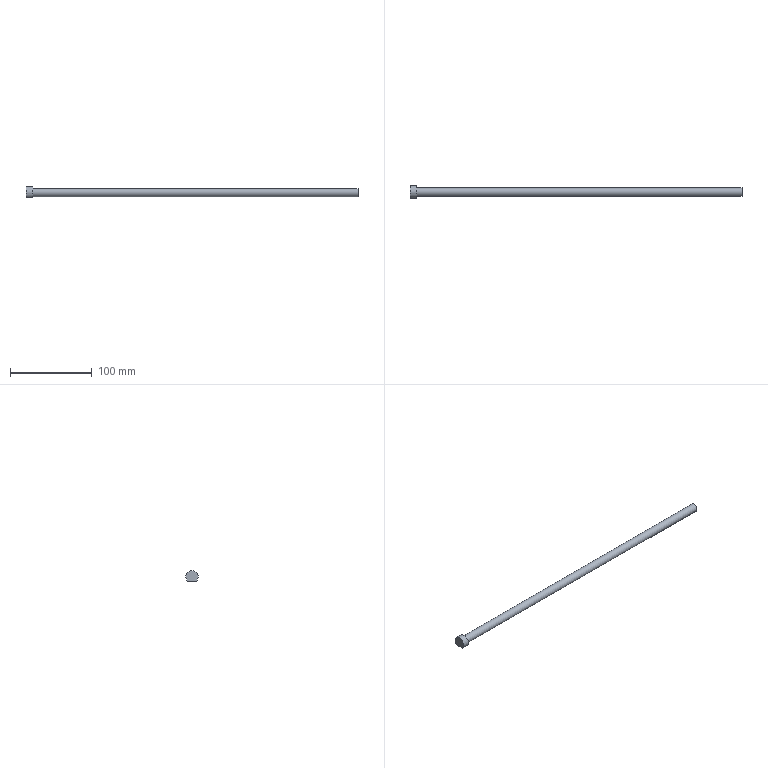Part | STEP file | solid 41 | 1 solid | 6 faces | box 405 x 15 x 13 mm | volume 32482 mm3 | plane 4 | cylinder 2 | commonest cylinder face diameters 10 x1 15 x1